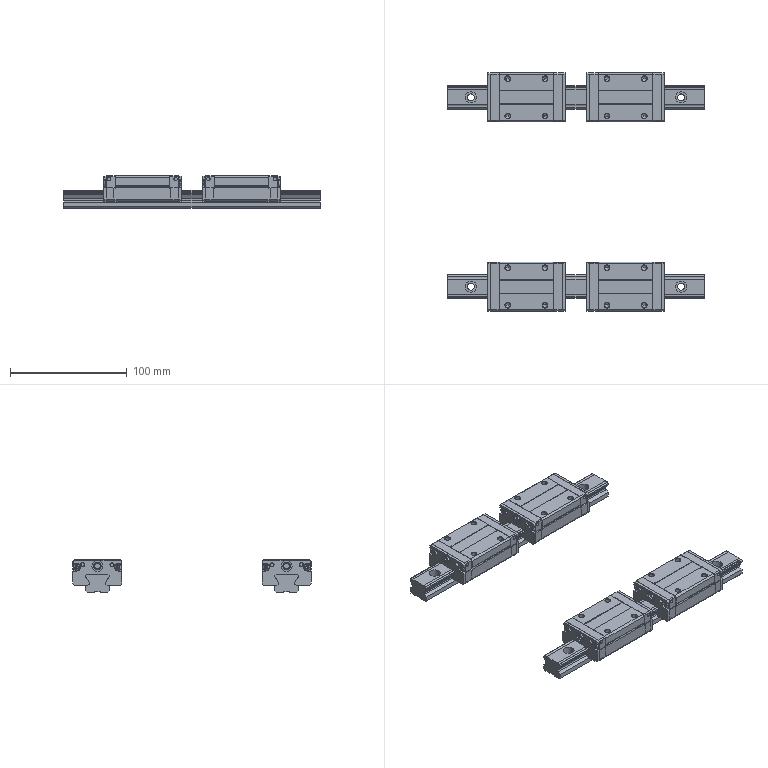Part | NX | 22 solids | 1716 faces | box 220 x 204 x 28 mm | volume 279610 mm3 | plane 984 | cylinder 572 | cone 128 | torus 32 | commonest cylinder face diameters 3 x96 3.5 x64 6.5 x64 4 x40 1.51 x32 3.4 x32